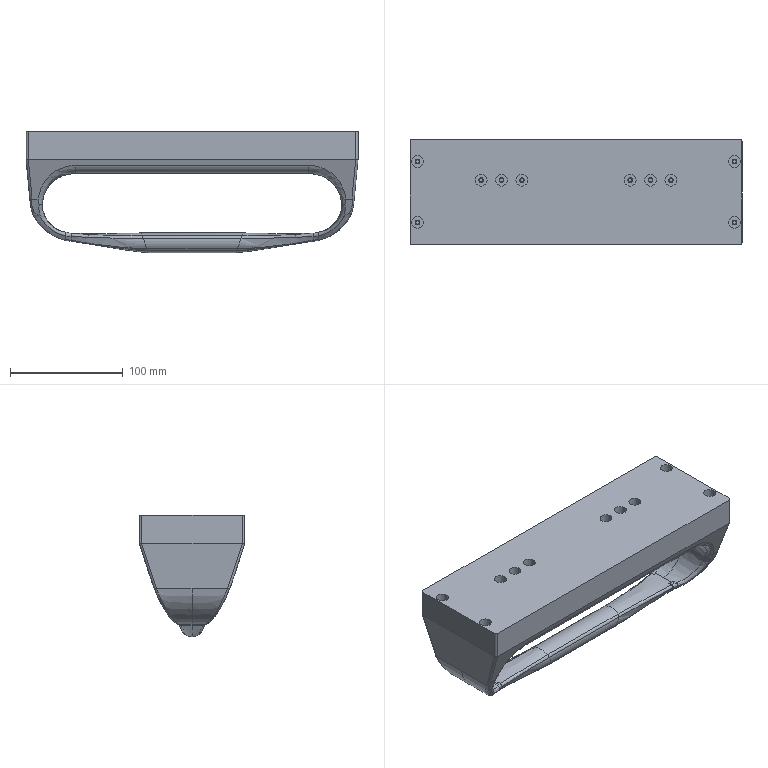NC program | NX | posted with a generic post | part box 294.078 x 93.5 x 107.5 mm
Lines 1 to 373 of 3753:
N10 G17 G21 G94 G90
(FLOOR_WALL , TOOL : D63)
N12 T01 M6
N14 G54
N16 G17 G0 G90 X-186.539 Y51.747 B0. C0. S6500 M3
N18 G43 Z28.5 H1
N20 Z3.
N22 G94 G1 Z0. F1250.
N24 X-183.539
N26 X183.539
N28 Y12.599
N30 X-183.539
N32 Y-26.55
N34 X183.539
N36 X186.539
N38 Z3.
N40 G0 Z28.5
N42 M5
(DRILLING_COPY_1 , TOOL : D6A45)
N44 T07 M6
N46 G54
N48 G17 G0 G90 X140.394 Y-27. B0. C0. S5000 M3
N50 G43 Z28.5 H7
N52 G94 G81 G98 Z-3.6 F250. R1.5
N54 Y27.
N56 X84.042 Y10.5 Z-2.1 R3.
N58 X66.042
N60 X48.042
N62 X-47.958
N64 X-65.958
N66 X-83.958
N68 X-140.394 Y27. Z-3.6 R1.5
N70 Y-27.
N72 G80
N74 G0 X-140.394 Y-27. Z28.5
N76 M5
(DRILLING_COPY_COPY_1 , TOOL : 3.2ZT)
N78 T13 M6
N80 G54
N82 G17 G0 G90 X140.394 Y-27. B0. C0. S2000 M3
N84 G43 Z28.5 H13
N86 G94 G83 G98 Z-12.961 F120. Q2. R1.5
N88 Y27.
N90 X84.042 Y10.5 Z-11.461 R3.
N92 X66.042
N94 X48.042
N96 X-47.958
N98 X-65.958
N100 X-83.958
N102 X-140.394 Y27. Z-12.961 R1.5
N104 Y-27.
N106 G80
N108 G0 X-140.394 Y-27. Z28.5
N110 M5
(FLOOR_WALL_1_1_COPY , TOOL : D10JING)
N112 T11 M6
N114 G54
N116 G17 G0 G90 X-146.792 Y53.04 B0. C0. S7500 M3
N118 G43 Z28.5 H11
N120 Z0.
N122 G94 G1 Z-1.5 F1250.
N124 X-146.336 Y52.25
N126 G3 X-145.47 Y51.75 R1.
N128 G1 X145.177
N130 G2 X151.737 Y46.776 R6.925
N132 G1 X-151.753
N134 X-151.761 Y46.759
N136 X-152.039 Y45.05
N138 Y41.802
N140 X152.039
N142 Y36.829
N144 X-152.039
N146 Y31.855
N148 X152.039
N150 Y26.881
N152 X131.395
N154 G3 X132.973 Y21.908 R9.
N156 G1 X152.039
N158 Y16.934
N160 X139.391
N162 X139.394 Y11.96
N164 X152.039
N166 Y6.987
N168 X139.394
N170 Y2.013
N172 X152.039
N174 Y-2.96
N176 X139.394
N178 Y-7.934
N180 X152.039
N182 Y-12.908
N184 X139.394
N186 X139.064 Y-17.881
N188 X152.039
N190 Y-22.855
N192 X132.405
N194 G3 X131.394 Y-27. R9.
N196 G1 Y-27.829
N198 X152.039
N200 G3 X152.905 Y-27.329 R1.
N202 G1 X153.539 Y-26.231
N204 Z0.
N206 G0 Z28.5
N208 X-129.894 Y28.481
N210 Z0.
N212 G1 Z-1.5
N214 X-130.529 Y27.381
N216 G2 X-131.395 Y26.881 R1.
N218 G1 X-152.039
N220 Y21.908
N222 X-132.973
N224 X-133.79 Y20.886
N226 X-134.746 Y19.993
N228 X-135.821 Y19.248
N230 X-139.391 Y16.934
N232 X-152.039
N234 Y11.96
N236 X-139.394
N238 Y6.987
N240 X-152.039
N242 Y2.013
N244 X-139.394
N246 Y-2.96
N248 X-152.039
N250 Y-7.934
N252 X-139.394
N254 Y-12.908
N256 X-152.039
N258 Y-17.881
N260 X-139.064
N262 X-137.024 Y-18.655
N264 G2 X-132.405 Y-22.855 R9.
N266 G1 X-152.039
N268 Y-27.829
N270 X-131.394
N272 G3 X-130.528 Y-27.329 R1.
N274 G1 X-129.919 Y-26.274
N276 Z0.
N278 G0 Z28.5
N280 X153.539 Y-31.204
N282 Z0.
N284 G1 Z-1.5
N286 X152.905 Y-32.302
N288 G2 X152.039 Y-32.802 R1.
N290 G1 X-152.039
N292 Y-37.776
N294 X152.039
N296 Y-42.75
N298 X-152.039
N300 G2 X-152.905 Y-42.25 R1.
N302 G1 X-153.539 Y-41.152
N304 Z0.
N306 G0 Z28.5
N308 X-129.583 Y30.144
N310 Z-9.5
N312 G1 Z-11.
N314 G3 X-130.449 Y30.644 R1.
N316 G1 X130.449
N318 G2 X130.894 Y30.147 R0.5
N320 G1 Y27.
N322 G3 X130.947 Y25.994 R9.5
N324 G1 X130.954 Y25.929
N326 X88.773
N328 G2 X94.928 Y21.215 R8.5
N330 G1 X132.859
N332 G3 X137.04 Y18.112 R9.5
N334 X137.434 Y17.976 R9.5
N336 G2 X137.984 Y17.198 R0.708
N338 G1 Y16.5
N340 X95.75
N342 Y11.785
N344 X137.984
N346 Y7.071
N348 X95.75
N350 Y3.
N352 G2 X95.726 Y2.356 R8.5
N354 G1 X137.984
N356 Y-2.359
N358 X93.848
N360 Z-9.5
N362 G0 Z28.5
N364 X-87.824 Y26.429
N366 Z-9.5
N368 G1 Z-11.
N370 G2 X-88.69 Y25.929 R1.
N372 G1 X-130.954
N374 G2 X-132.859 Y21.215 R9.5
N376 G1 X-94.844
N378 G3 X-95.667 Y17.567 R8.5
N380 G1 Y16.5
N382 X-137.984
N384 Y11.785
N386 X-95.667
N388 Y7.071
N390 X-137.984
N392 Y2.356
N394 X-95.642
N396 G3 X-93.765 Y-2.359 R8.5
N398 G1 X-137.984
N400 Z-9.5
N402 G0 Z28.5
N404 X45.593 Y26.429
N406 Z-9.5
N408 G1 Z-11.
N410 G2 X44.727 Y25.929 R1.
N412 G1 X-44.644
N414 G2 X-38.489 Y21.215 R8.5
N416 G1 X38.573
N418 G3 X37.75 Y17.567 R8.5
N420 G1 Y16.5
N422 X4.614
N424 X1.884 Y11.785
N426 X37.75
N428 G3 X37.25 Y12.651 R1.
N430 G1 Z-9.5
N432 G0 Z28.5
N434 X-3.665 Y17.
N436 Z-9.5
N438 G1 Z-11.
N440 G2 X-4.531 Y16.5 R1.
N442 G1 X-37.667
N444 Y11.785
N446 X-1.801
N448 G3 X-0.935 Y12.285 R1.
N450 G1 Z-9.5
N452 G0 Z28.5
N454 X37.75 Y11.785
N456 Z-9.5
N458 G1 Z-11.
N460 Y7.071
N462 X-37.667
N464 Y3.
N466 G2 X-37.691 Y2.356 R8.5
N468 G1 X37.774
N470 G3 X39.652 Y-2.359 R8.5
N472 G1 X-39.569
N474 Z-9.5
N476 G0 Z28.5
N478 X-137.484 Y-6.208
N480 Z-9.5
N482 G1 Z-11.
N484 G3 X-137.984 Y-7.074 R1.
N486 G1 X137.984
N488 Y-11.788
N490 X-137.984
N492 Y-16.503
N494 X137.984
N496 Y-17.236
N498 X137.985 Y-17.269
N500 G2 X137.686 Y-17.861 R0.649
N502 G1 X137.315 Y-18.013
N504 G3 X132.856 Y-21.218 R9.5
N506 G1 X-132.856
N508 G2 X-130.954 Y-25.932 R9.5
N510 G1 X130.954
N512 X130.947 Y-25.994
N514 G3 X130.894 Y-27. R9.5
N516 G1 Y-30.147
N518 G2 X130.399 Y-30.647 R0.5
N520 G1 X-130.399
N522 G2 X-130.832 Y-30.397 R0.5
N524 G1 X-131.265 Y-30.638
N526 G3 X-130.404 Y-31.147 R1.
N528 G1 X130.394
N530 G3 X131.394 Y-30.147 R1.
N532 G1 Y-27.
N534 G2 X137.491 Y-18.481 R9.
N536 G1 X137.911 Y-18.309
N538 G3 X138.484 Y-17.236 R1.149
N540 G1 Y17.198
N542 G3 X137.541 Y18.464 R1.206
N544 G2 X131.394 Y27. R9.
N546 G1 Y30.147
N548 G3 X130.394 Y31.147 R1.
N550 G1 X-130.394
N552 G3 X-131.394 Y30.147 R1.
N554 G1 Y27.
N556 G2 X-137.491 Y18.481 R9.
N558 G1 X-137.911 Y18.309
N560 G3 X-138.484 Y17.236 R1.149
N562 G1 Y-17.208
N564 G3 X-137.706 Y-18.411 R1.185
N566 G2 X-131.394 Y-27. R9.
N568 G1 Y-30.147
N570 G3 X-130.404 Y-31.147 R1.
N572 X-129.533 Y-30.656 R1.
N574 G1 X-128.937 Y-29.647
N576 Z-9.5
N578 G0 Z28.5
N580 X-64.935 Y-7.
N582 Z-9.5
N584 G1 Z-11.
N586 X-65.801 Y-5.5
N588 G3 X-66.667 Y-5. R1.
N590 G1 X-87.167
N592 G2 X-95.167 Y3. R8.
N594 G1 Y17.567
N596 G2 X-87.167 Y25.567 R8.
N598 G1 X-46.167
N600 G2 X-38.167 Y17.567 R8.
N602 G1 Y3.
N604 G2 X-46.167 Y-5. R8.
N606 G1 X-66.667
N608 G3 X-67.533 Y-5.5 R1.
N610 G1 X-68.399 Y-7.
N612 Z-9.5
N614 G0 Z28.5
N616 X65.018 Y27.567
N618 Z-9.5
N620 G1 Z-11.
N622 X65.884 Y26.067
N624 G3 X66.75 Y25.567 R1.
N626 G1 X87.25
N628 G2 X95.25 Y17.567 R8.
N630 G1 Y3.
N632 G2 X87.25 Y-5. R8.
N634 G1 X46.25
N636 G2 X38.25 Y3. R8.
N638 G1 Y17.567
N640 G2 X46.25 Y25.567 R8.
N642 G1 X66.75
N644 G3 X67.616 Y26.067 R1.
N646 G1 X68.482 Y27.567
N648 Z-9.5
N650 G0 Z28.5
(ZLEVEL_PROFILE_COPY_COPY_1_COPY_COPY_COPY , TOOL : D10JING)
N652 X146.126 Y-52.672
N654 Z-18.5
N656 G1 Z-21.5 F1000.
N658 X145.883 Y-52.25
N660 G3 X145.017 Y-51.75 R1.
N662 G1 X-145.017
N664 G2 X-151.747 Y-46.671 R7.017
N666 X-152.039 Y-44.64 R7.514
N668 G1 Y44.641
N670 G2 X-150.152 Y49.502 R7.2
N672 X-145.024 Y51.75 R6.989
N674 G1 X144.965
N676 G2 X152.039 Y44.686 R7.049
N678 G1 Y-44.646
N680 G2 X149.351 Y-50.244 R7.149
N682 X145.017 Y-51.75 R7.007
N684 G3 X144.151 Y-52.251 R1.
N686 G1 X143.863 Y-52.75
N688 Z-18.5
N690 G0 Z28.5
(ZLEVEL_PROFILE_COPY_COPY_1_COPY_COPY_COPY_COPY , TOOL : D10JING)
N692 X1.335 Y19.36
N694 Z-10.5
N696 G1 Z-13.5
N698 X0.908 Y20.1
N700 G3 X0.042 Y20.6 R1.
N702 X-4.558 Y16. R4.6
N704 X0.042 Y20.6 R-4.6
N706 X-0.824 Y20.1 R1.
N708 G1 X-1.252 Y19.36
N710 Z-10.5
N712 G0 Z28.5
N714 M5